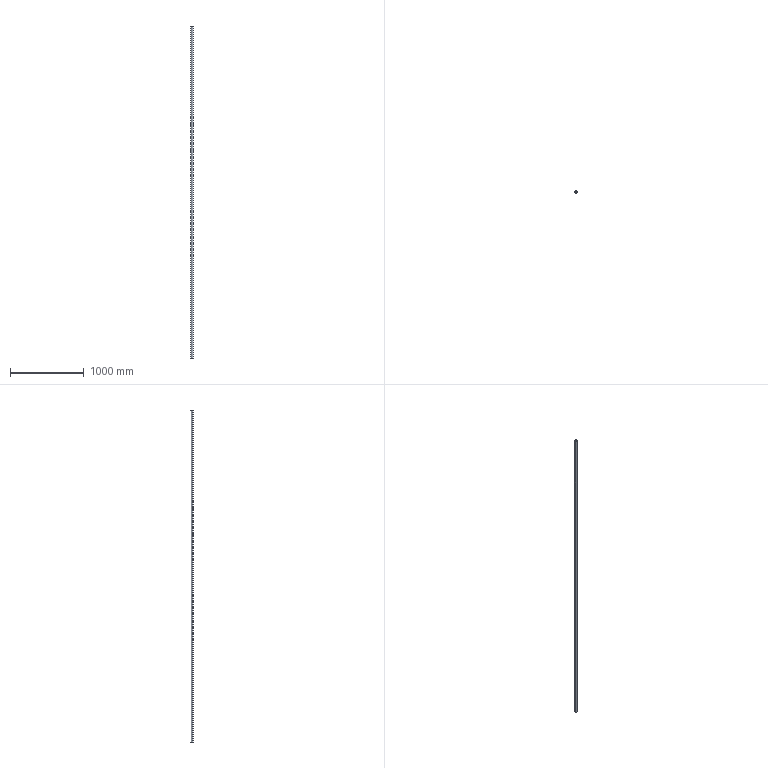Part | SolidWorks | features Extrusion 1 | 1 solid | 6 faces | box 35 x 35 x 4500 mm | volume 1357168 mm3 | cylinder 4 | plane 2 | commonest cylinder face diameters 29 x2 35 x2
STEP:
#1=CARTESIAN_POINT('',(-14.5,0.,4500.));
#2=VERTEX_POINT('',#1);
#3=CARTESIAN_POINT('',(14.5,0.,4500.));
#4=VERTEX_POINT('',#3);
#5=CARTESIAN_POINT('',(0.,0.,4500.));
#6=DIRECTION('',(0.,0.,1.));
#7=DIRECTION('',(1.,0.,0.));
#8=AXIS2_PLACEMENT_3D('',#5,#6,#7);
#9=CIRCLE('',#8,14.5);
#10=EDGE_CURVE('',#2,#4,#9,.T.);
#11=ORIENTED_EDGE('',*,*,#10,.T.);
#12=CARTESIAN_POINT('',(14.5,0.,0.));
#13=VERTEX_POINT('',#12);
#14=CARTESIAN_POINT('',(14.5,0.,4500.));
#15=DIRECTION('',(0.,0.,-1.));
#16=VECTOR('',#15,1000.);
#17=LINE('',#14,#16);
#18=EDGE_CURVE('',#4,#13,#17,.T.);
#19=ORIENTED_EDGE('',*,*,#18,.T.);
#20=CARTESIAN_POINT('',(-14.5,0.,0.));
#21=VERTEX_POINT('',#20);
#22=CARTESIAN_POINT('',(0.,0.,0.));
#23=DIRECTION('',(0.,0.,1.));
#24=DIRECTION('',(1.,0.,0.));
#25=AXIS2_PLACEMENT_3D('',#22,#23,#24);
#26=CIRCLE('',#25,14.5);
#27=EDGE_CURVE('',#21,#13,#26,.T.);
#28=ORIENTED_EDGE('',*,*,#27,.F.);
#29=CARTESIAN_POINT('',(-14.5,0.,4500.));
#30=DIRECTION('',(0.,0.,-1.));
#31=VECTOR('',#30,1000.);
#32=LINE('',#29,#31);
#33=EDGE_CURVE('',#2,#21,#32,.T.);
#34=ORIENTED_EDGE('',*,*,#33,.F.);
#35=EDGE_LOOP('',(#11,#19,#28,#34));
#36=FACE_OUTER_BOUND('',#35,.T.);
#37=CARTESIAN_POINT('',(0.,0.,4500.));
#38=DIRECTION('',(0.,0.,-1.));
#39=DIRECTION('',(-1.,0.,0.));
#40=AXIS2_PLACEMENT_3D('',#37,#38,#39);
#41=CYLINDRICAL_SURFACE('',#40,14.5);
#42=ADVANCED_FACE('',(#36),#41,.F.);
#43=CARTESIAN_POINT('',(17.5,0.,4500.));
#44=VERTEX_POINT('',#43);
#45=CARTESIAN_POINT('',(-17.5,0.,4500.));
#46=VERTEX_POINT('',#45);
#47=CARTESIAN_POINT('',(0.,0.,4500.));
#48=DIRECTION('',(0.,0.,1.));
#49=DIRECTION('',(1.,0.,0.));
#50=AXIS2_PLACEMENT_3D('',#47,#48,#49);
#51=CIRCLE('',#50,17.5);
#52=EDGE_CURVE('',#44,#46,#51,.T.);
#53=ORIENTED_EDGE('',*,*,#52,.F.);
#54=CARTESIAN_POINT('',(17.5,0.,0.));
#55=VERTEX_POINT('',#54);
#56=CARTESIAN_POINT('',(17.5,0.,4500.));
#57=DIRECTION('',(0.,0.,-1.));
#58=VECTOR('',#57,1000.);
#59=LINE('',#56,#58);
#60=EDGE_CURVE('',#44,#55,#59,.T.);
#61=ORIENTED_EDGE('',*,*,#60,.T.);
#62=CARTESIAN_POINT('',(-17.5,0.,0.));
#63=VERTEX_POINT('',#62);
#64=CARTESIAN_POINT('',(0.,0.,0.));
#65=DIRECTION('',(0.,0.,1.));
#66=DIRECTION('',(1.,0.,0.));
#67=AXIS2_PLACEMENT_3D('',#64,#65,#66);
#68=CIRCLE('',#67,17.5);
#69=EDGE_CURVE('',#55,#63,#68,.T.);
#70=ORIENTED_EDGE('',*,*,#69,.T.);
#71=CARTESIAN_POINT('',(-17.5,0.,4500.));
#72=DIRECTION('',(0.,0.,-1.));
#73=VECTOR('',#72,1000.);
#74=LINE('',#71,#73);
#75=EDGE_CURVE('',#46,#63,#74,.T.);
#76=ORIENTED_EDGE('',*,*,#75,.F.);
#77=EDGE_LOOP('',(#53,#61,#70,#76));
#78=FACE_OUTER_BOUND('',#77,.T.);
#79=CARTESIAN_POINT('',(0.,0.,4500.));
#80=DIRECTION('',(0.,0.,-1.));
#81=DIRECTION('',(-1.,0.,0.));
#82=AXIS2_PLACEMENT_3D('',#79,#80,#81);
#83=CYLINDRICAL_SURFACE('',#82,17.5);
#84=ADVANCED_FACE('',(#78),#83,.T.);
#85=CARTESIAN_POINT('',(0.,0.,4500.));
#86=DIRECTION('',(0.,0.,1.));
#87=DIRECTION('',(1.,0.,0.));
#88=AXIS2_PLACEMENT_3D('',#85,#86,#87);
#89=CIRCLE('',#88,17.5);
#90=EDGE_CURVE('',#46,#44,#89,.T.);
#91=ORIENTED_EDGE('',*,*,#90,.T.);
#92=ORIENTED_EDGE('',*,*,#52,.T.);
#93=EDGE_LOOP('',(#91,#92));
#94=FACE_OUTER_BOUND('',#93,.T.);
#95=ORIENTED_EDGE('',*,*,#10,.F.);
#96=CARTESIAN_POINT('',(0.,0.,4500.));
#97=DIRECTION('',(0.,0.,1.));
#98=DIRECTION('',(1.,0.,0.));
#99=AXIS2_PLACEMENT_3D('',#96,#97,#98);
#100=CIRCLE('',#99,14.5);
#101=EDGE_CURVE('',#4,#2,#100,.T.);
#102=ORIENTED_EDGE('',*,*,#101,.F.);
#103=EDGE_LOOP('',(#95,#102));
#104=FACE_BOUND('',#103,.T.);
#105=CARTESIAN_POINT('',(0.,0.,4500.));
#106=DIRECTION('',(0.,0.,1.));
#107=DIRECTION('',(1.,0.,0.));
#108=AXIS2_PLACEMENT_3D('',#105,#106,#107);
#109=PLANE('',#108);
#110=ADVANCED_FACE('',(#94,#104),#109,.T.);
#111=CARTESIAN_POINT('',(0.,0.,0.));
#112=DIRECTION('',(0.,0.,1.));
#113=DIRECTION('',(1.,0.,0.));
#114=AXIS2_PLACEMENT_3D('',#111,#112,#113);
#115=CIRCLE('',#114,17.5);
#116=EDGE_CURVE('',#63,#55,#115,.T.);
#117=ORIENTED_EDGE('',*,*,#116,.F.);
#118=ORIENTED_EDGE('',*,*,#69,.F.);
#119=EDGE_LOOP('',(#117,#118));
#120=FACE_OUTER_BOUND('',#119,.T.);
#121=ORIENTED_EDGE('',*,*,#27,.T.);
#122=CARTESIAN_POINT('',(0.,0.,0.));
#123=DIRECTION('',(0.,0.,1.));
#124=DIRECTION('',(1.,0.,0.));
#125=AXIS2_PLACEMENT_3D('',#122,#123,#124);
#126=CIRCLE('',#125,14.5);
#127=EDGE_CURVE('',#13,#21,#126,.T.);
#128=ORIENTED_EDGE('',*,*,#127,.T.);
#129=EDGE_LOOP('',(#121,#128));
#130=FACE_BOUND('',#129,.T.);
#131=CARTESIAN_POINT('',(0.,0.,0.));
#132=DIRECTION('',(0.,0.,1.));
#133=DIRECTION('',(1.,0.,0.));
#134=AXIS2_PLACEMENT_3D('',#131,#132,#133);
#135=PLANE('',#134);
#136=ADVANCED_FACE('',(#120,#130),#135,.F.);
#137=ORIENTED_EDGE('',*,*,#60,.F.);
#138=ORIENTED_EDGE('',*,*,#90,.F.);
#139=ORIENTED_EDGE('',*,*,#75,.T.);
#140=ORIENTED_EDGE('',*,*,#116,.T.);
#141=EDGE_LOOP('',(#137,#138,#139,#140));
#142=FACE_OUTER_BOUND('',#141,.T.);
#143=CARTESIAN_POINT('',(0.,0.,4500.));
#144=DIRECTION('',(0.,0.,-1.));
#145=DIRECTION('',(-1.,0.,0.));
#146=AXIS2_PLACEMENT_3D('',#143,#144,#145);
#147=CYLINDRICAL_SURFACE('',#146,17.5);
#148=ADVANCED_FACE('',(#142),#147,.T.);
#149=ORIENTED_EDGE('',*,*,#18,.F.);
#150=ORIENTED_EDGE('',*,*,#101,.T.);
#151=ORIENTED_EDGE('',*,*,#33,.T.);
#152=ORIENTED_EDGE('',*,*,#127,.F.);
#153=EDGE_LOOP('',(#149,#150,#151,#152));
#154=FACE_OUTER_BOUND('',#153,.T.);
#155=CARTESIAN_POINT('',(0.,0.,4500.));
#156=DIRECTION('',(0.,0.,-1.));
#157=DIRECTION('',(-1.,0.,0.));
#158=AXIS2_PLACEMENT_3D('',#155,#156,#157);
#159=CYLINDRICAL_SURFACE('',#158,14.5);
#160=ADVANCED_FACE('',(#154),#159,.F.);
#161=CLOSED_SHELL('',(#42,#84,#110,#136,#148,#160));
#162=MANIFOLD_SOLID_BREP('',#161);
#163=CARTESIAN_POINT('',(0.,0.,0.));
#164=DIRECTION('',(0.,0.,1.));
#165=DIRECTION('',(1.,0.,0.));
#166=AXIS2_PLACEMENT_3D('',#163,#164,#165);
#167=(LENGTH_UNIT()NAMED_UNIT(*)SI_UNIT(.MILLI.,.METRE.));
#168=UNCERTAINTY_MEASURE_WITH_UNIT(LENGTH_MEASURE(0.00001),#167,'','');
#169=(NAMED_UNIT(*)PLANE_ANGLE_UNIT()SI_UNIT($,.RADIAN.));
#170=(NAMED_UNIT(*)SI_UNIT($,.STERADIAN.)SOLID_ANGLE_UNIT());
#171=(GEOMETRIC_REPRESENTATION_CONTEXT(3)GLOBAL_UNCERTAINTY_ASSIGNED_CONTEXT((#168))GLOBAL_UNIT_ASSIGNED_CONTEXT((#167,#169,#170))REPRESENTATION_CONTEXT('',''));
#172=ADVANCED_BREP_SHAPE_REPRESENTATION('',(#162,#166),#171);